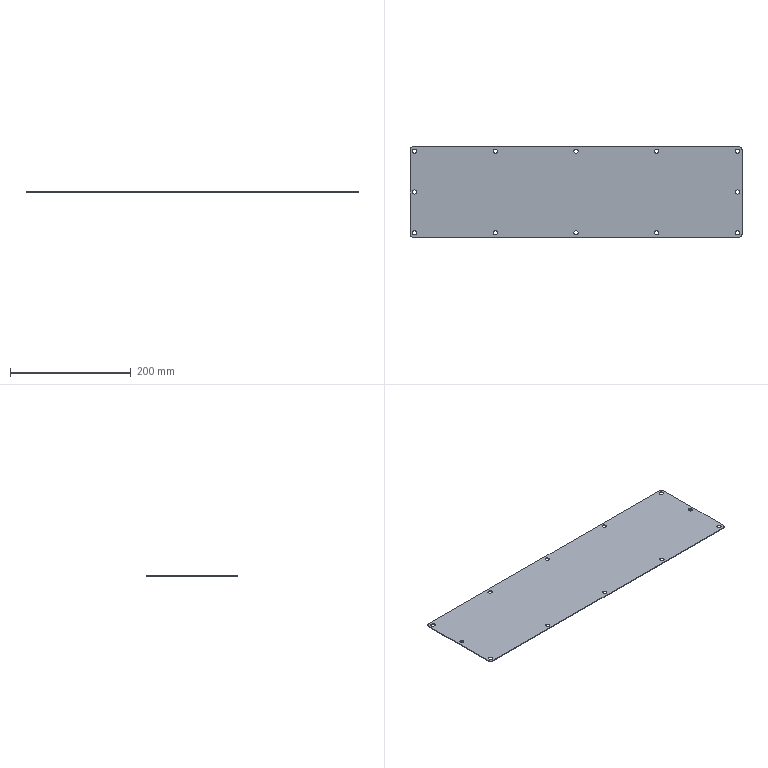Part | SolidWorks | features FlatPattern 1, SMBaseFlange 1, SheetMetal 1 | 1 solid | 34 faces | box 550 x 150 x 1.2 mm | volume 98420 mm3 | cylinder 28 | plane 6 | commonest cylinder face diameters 7 x24 10 x4
STEP:
#1=CARTESIAN_POINT('',(264.,7.5,1.2));
#2=VERTEX_POINT('',#1);
#3=CARTESIAN_POINT('',(271.,7.5,1.2));
#4=VERTEX_POINT('',#3);
#5=CARTESIAN_POINT('',(267.5,7.5,1.2));
#6=DIRECTION('',(0.,0.,1.));
#7=DIRECTION('',(1.,0.,0.));
#8=AXIS2_PLACEMENT_3D('',#5,#6,#7);
#9=CIRCLE('',#8,3.5);
#10=EDGE_CURVE('',#2,#4,#9,.T.);
#11=ORIENTED_EDGE('',*,*,#10,.T.);
#12=CARTESIAN_POINT('',(271.,7.5,0.));
#13=VERTEX_POINT('',#12);
#14=CARTESIAN_POINT('',(271.,7.5,1.2));
#15=DIRECTION('',(0.,0.,-1.));
#16=VECTOR('',#15,1000.);
#17=LINE('',#14,#16);
#18=EDGE_CURVE('',#4,#13,#17,.T.);
#19=ORIENTED_EDGE('',*,*,#18,.T.);
#20=CARTESIAN_POINT('',(264.,7.5,0.));
#21=VERTEX_POINT('',#20);
#22=CARTESIAN_POINT('',(267.5,7.5,0.));
#23=DIRECTION('',(0.,0.,1.));
#24=DIRECTION('',(1.,0.,0.));
#25=AXIS2_PLACEMENT_3D('',#22,#23,#24);
#26=CIRCLE('',#25,3.5);
#27=EDGE_CURVE('',#21,#13,#26,.T.);
#28=ORIENTED_EDGE('',*,*,#27,.F.);
#29=CARTESIAN_POINT('',(264.,7.5,1.2));
#30=DIRECTION('',(0.,0.,-1.));
#31=VECTOR('',#30,1000.);
#32=LINE('',#29,#31);
#33=EDGE_CURVE('',#2,#21,#32,.T.);
#34=ORIENTED_EDGE('',*,*,#33,.F.);
#35=EDGE_LOOP('',(#11,#19,#28,#34));
#36=FACE_OUTER_BOUND('',#35,.T.);
#37=CARTESIAN_POINT('',(267.5,7.5,1.2));
#38=DIRECTION('',(0.,0.,-1.));
#39=DIRECTION('',(-1.,0.,0.));
#40=AXIS2_PLACEMENT_3D('',#37,#38,#39);
#41=CYLINDRICAL_SURFACE('',#40,3.5);
#42=ADVANCED_FACE('',(#36),#41,.F.);
#43=CARTESIAN_POINT('',(264.,142.5,1.2));
#44=VERTEX_POINT('',#43);
#45=CARTESIAN_POINT('',(271.,142.5,1.2));
#46=VERTEX_POINT('',#45);
#47=CARTESIAN_POINT('',(267.5,142.5,1.2));
#48=DIRECTION('',(0.,0.,1.));
#49=DIRECTION('',(1.,0.,0.));
#50=AXIS2_PLACEMENT_3D('',#47,#48,#49);
#51=CIRCLE('',#50,3.5);
#52=EDGE_CURVE('',#44,#46,#51,.T.);
#53=ORIENTED_EDGE('',*,*,#52,.T.);
#54=CARTESIAN_POINT('',(271.,142.5,0.));
#55=VERTEX_POINT('',#54);
#56=CARTESIAN_POINT('',(271.,142.5,1.2));
#57=DIRECTION('',(0.,0.,-1.));
#58=VECTOR('',#57,1000.);
#59=LINE('',#56,#58);
#60=EDGE_CURVE('',#46,#55,#59,.T.);
#61=ORIENTED_EDGE('',*,*,#60,.T.);
#62=CARTESIAN_POINT('',(264.,142.5,0.));
#63=VERTEX_POINT('',#62);
#64=CARTESIAN_POINT('',(267.5,142.5,0.));
#65=DIRECTION('',(0.,0.,1.));
#66=DIRECTION('',(1.,0.,0.));
#67=AXIS2_PLACEMENT_3D('',#64,#65,#66);
#68=CIRCLE('',#67,3.5);
#69=EDGE_CURVE('',#63,#55,#68,.T.);
#70=ORIENTED_EDGE('',*,*,#69,.F.);
#71=CARTESIAN_POINT('',(264.,142.5,1.2));
#72=DIRECTION('',(0.,0.,-1.));
#73=VECTOR('',#72,1000.);
#74=LINE('',#71,#73);
#75=EDGE_CURVE('',#44,#63,#74,.T.);
#76=ORIENTED_EDGE('',*,*,#75,.F.);
#77=EDGE_LOOP('',(#53,#61,#70,#76));
#78=FACE_OUTER_BOUND('',#77,.T.);
#79=CARTESIAN_POINT('',(267.5,142.5,1.2));
#80=DIRECTION('',(0.,0.,-1.));
#81=DIRECTION('',(-1.,0.,0.));
#82=AXIS2_PLACEMENT_3D('',#79,#80,#81);
#83=CYLINDRICAL_SURFACE('',#82,3.5);
#84=ADVANCED_FACE('',(#78),#83,.F.);
#85=CARTESIAN_POINT('',(130.25,7.5,1.2));
#86=VERTEX_POINT('',#85);
#87=CARTESIAN_POINT('',(137.25,7.5,1.2));
#88=VERTEX_POINT('',#87);
#89=CARTESIAN_POINT('',(133.75,7.5,1.2));
#90=DIRECTION('',(0.,0.,1.));
#91=DIRECTION('',(1.,0.,0.));
#92=AXIS2_PLACEMENT_3D('',#89,#90,#91);
#93=CIRCLE('',#92,3.5);
#94=EDGE_CURVE('',#86,#88,#93,.T.);
#95=ORIENTED_EDGE('',*,*,#94,.T.);
#96=CARTESIAN_POINT('',(137.25,7.5,0.));
#97=VERTEX_POINT('',#96);
#98=CARTESIAN_POINT('',(137.25,7.5,1.2));
#99=DIRECTION('',(0.,0.,-1.));
#100=VECTOR('',#99,1000.);
#101=LINE('',#98,#100);
#102=EDGE_CURVE('',#88,#97,#101,.T.);
#103=ORIENTED_EDGE('',*,*,#102,.T.);
#104=CARTESIAN_POINT('',(130.25,7.5,0.));
#105=VERTEX_POINT('',#104);
#106=CARTESIAN_POINT('',(133.75,7.5,0.));
#107=DIRECTION('',(0.,0.,1.));
#108=DIRECTION('',(1.,0.,0.));
#109=AXIS2_PLACEMENT_3D('',#106,#107,#108);
#110=CIRCLE('',#109,3.5);
#111=EDGE_CURVE('',#105,#97,#110,.T.);
#112=ORIENTED_EDGE('',*,*,#111,.F.);
#113=CARTESIAN_POINT('',(130.25,7.5,1.2));
#114=DIRECTION('',(0.,0.,-1.));
#115=VECTOR('',#114,1000.);
#116=LINE('',#113,#115);
#117=EDGE_CURVE('',#86,#105,#116,.T.);
#118=ORIENTED_EDGE('',*,*,#117,.F.);
#119=EDGE_LOOP('',(#95,#103,#112,#118));
#120=FACE_OUTER_BOUND('',#119,.T.);
#121=CARTESIAN_POINT('',(133.75,7.5,1.2));
#122=DIRECTION('',(0.,0.,-1.));
#123=DIRECTION('',(-1.,0.,0.));
#124=AXIS2_PLACEMENT_3D('',#121,#122,#123);
#125=CYLINDRICAL_SURFACE('',#124,3.5);
#126=ADVANCED_FACE('',(#120),#125,.F.);
#127=CARTESIAN_POINT('',(130.25,142.5,1.2));
#128=VERTEX_POINT('',#127);
#129=CARTESIAN_POINT('',(137.25,142.5,1.2));
#130=VERTEX_POINT('',#129);
#131=CARTESIAN_POINT('',(133.75,142.5,1.2));
#132=DIRECTION('',(0.,0.,1.));
#133=DIRECTION('',(1.,0.,0.));
#134=AXIS2_PLACEMENT_3D('',#131,#132,#133);
#135=CIRCLE('',#134,3.5);
#136=EDGE_CURVE('',#128,#130,#135,.T.);
#137=ORIENTED_EDGE('',*,*,#136,.T.);
#138=CARTESIAN_POINT('',(137.25,142.5,0.));
#139=VERTEX_POINT('',#138);
#140=CARTESIAN_POINT('',(137.25,142.5,1.2));
#141=DIRECTION('',(0.,0.,-1.));
#142=VECTOR('',#141,1000.);
#143=LINE('',#140,#142);
#144=EDGE_CURVE('',#130,#139,#143,.T.);
#145=ORIENTED_EDGE('',*,*,#144,.T.);
#146=CARTESIAN_POINT('',(130.25,142.5,0.));
#147=VERTEX_POINT('',#146);
#148=CARTESIAN_POINT('',(133.75,142.5,0.));
#149=DIRECTION('',(0.,0.,1.));
#150=DIRECTION('',(1.,0.,0.));
#151=AXIS2_PLACEMENT_3D('',#148,#149,#150);
#152=CIRCLE('',#151,3.5);
#153=EDGE_CURVE('',#147,#139,#152,.T.);
#154=ORIENTED_EDGE('',*,*,#153,.F.);
#155=CARTESIAN_POINT('',(130.25,142.5,1.2));
#156=DIRECTION('',(0.,0.,-1.));
#157=VECTOR('',#156,1000.);
#158=LINE('',#155,#157);
#159=EDGE_CURVE('',#128,#147,#158,.T.);
#160=ORIENTED_EDGE('',*,*,#159,.F.);
#161=EDGE_LOOP('',(#137,#145,#154,#160));
#162=FACE_OUTER_BOUND('',#161,.T.);
#163=CARTESIAN_POINT('',(133.75,142.5,1.2));
#164=DIRECTION('',(0.,0.,-1.));
#165=DIRECTION('',(-1.,0.,0.));
#166=AXIS2_PLACEMENT_3D('',#163,#164,#165);
#167=CYLINDRICAL_SURFACE('',#166,3.5);
#168=ADVANCED_FACE('',(#162),#167,.F.);
#169=CARTESIAN_POINT('',(-3.5,7.5,1.2));
#170=VERTEX_POINT('',#169);
#171=CARTESIAN_POINT('',(3.5,7.5,1.2));
#172=VERTEX_POINT('',#171);
#173=CARTESIAN_POINT('',(0.,7.5,1.2));
#174=DIRECTION('',(0.,0.,1.));
#175=DIRECTION('',(1.,0.,0.));
#176=AXIS2_PLACEMENT_3D('',#173,#174,#175);
#177=CIRCLE('',#176,3.5);
#178=EDGE_CURVE('',#170,#172,#177,.T.);
#179=ORIENTED_EDGE('',*,*,#178,.T.);
#180=CARTESIAN_POINT('',(3.5,7.5,0.));
#181=VERTEX_POINT('',#180);
#182=CARTESIAN_POINT('',(3.5,7.5,1.2));
#183=DIRECTION('',(0.,0.,-1.));
#184=VECTOR('',#183,1000.);
#185=LINE('',#182,#184);
#186=EDGE_CURVE('',#172,#181,#185,.T.);
#187=ORIENTED_EDGE('',*,*,#186,.T.);
#188=CARTESIAN_POINT('',(-3.5,7.5,0.));
#189=VERTEX_POINT('',#188);
#190=CARTESIAN_POINT('',(0.,7.5,0.));
#191=DIRECTION('',(0.,0.,1.));
#192=DIRECTION('',(1.,0.,0.));
#193=AXIS2_PLACEMENT_3D('',#190,#191,#192);
#194=CIRCLE('',#193,3.5);
#195=EDGE_CURVE('',#189,#181,#194,.T.);
#196=ORIENTED_EDGE('',*,*,#195,.F.);
#197=CARTESIAN_POINT('',(-3.5,7.5,1.2));
#198=DIRECTION('',(0.,0.,-1.));
#199=VECTOR('',#198,1000.);
#200=LINE('',#197,#199);
#201=EDGE_CURVE('',#170,#189,#200,.T.);
#202=ORIENTED_EDGE('',*,*,#201,.F.);
#203=EDGE_LOOP('',(#179,#187,#196,#202));
#204=FACE_OUTER_BOUND('',#203,.T.);
#205=CARTESIAN_POINT('',(0.,7.5,1.2));
#206=DIRECTION('',(0.,0.,-1.));
#207=DIRECTION('',(-1.,0.,0.));
#208=AXIS2_PLACEMENT_3D('',#205,#206,#207);
#209=CYLINDRICAL_SURFACE('',#208,3.5);
#210=ADVANCED_FACE('',(#204),#209,.F.);
#211=CARTESIAN_POINT('',(-3.5,142.5,1.2));
#212=VERTEX_POINT('',#211);
#213=CARTESIAN_POINT('',(3.5,142.5,1.2));
#214=VERTEX_POINT('',#213);
#215=CARTESIAN_POINT('',(0.,142.5,1.2));
#216=DIRECTION('',(0.,0.,1.));
#217=DIRECTION('',(1.,0.,0.));
#218=AXIS2_PLACEMENT_3D('',#215,#216,#217);
#219=CIRCLE('',#218,3.5);
#220=EDGE_CURVE('',#212,#214,#219,.T.);
#221=ORIENTED_EDGE('',*,*,#220,.T.);
#222=CARTESIAN_POINT('',(3.5,142.5,0.));
#223=VERTEX_POINT('',#222);
#224=CARTESIAN_POINT('',(3.5,142.5,1.2));
#225=DIRECTION('',(0.,0.,-1.));
#226=VECTOR('',#225,1000.);
#227=LINE('',#224,#226);
#228=EDGE_CURVE('',#214,#223,#227,.T.);
#229=ORIENTED_EDGE('',*,*,#228,.T.);
#230=CARTESIAN_POINT('',(-3.5,142.5,0.));
#231=VERTEX_POINT('',#230);
#232=CARTESIAN_POINT('',(0.,142.5,0.));
#233=DIRECTION('',(0.,0.,1.));
#234=DIRECTION('',(1.,0.,0.));
#235=AXIS2_PLACEMENT_3D('',#232,#233,#234);
#236=CIRCLE('',#235,3.5);
#237=EDGE_CURVE('',#231,#223,#236,.T.);
#238=ORIENTED_EDGE('',*,*,#237,.F.);
#239=CARTESIAN_POINT('',(-3.5,142.5,1.2));
#240=DIRECTION('',(0.,0.,-1.));
#241=VECTOR('',#240,1000.);
#242=LINE('',#239,#241);
#243=EDGE_CURVE('',#212,#231,#242,.T.);
#244=ORIENTED_EDGE('',*,*,#243,.F.);
#245=EDGE_LOOP('',(#221,#229,#238,#244));
#246=FACE_OUTER_BOUND('',#245,.T.);
#247=CARTESIAN_POINT('',(0.,142.5,1.2));
#248=DIRECTION('',(0.,0.,-1.));
#249=DIRECTION('',(-1.,0.,0.));
#250=AXIS2_PLACEMENT_3D('',#247,#248,#249);
#251=CYLINDRICAL_SURFACE('',#250,3.5);
#252=ADVANCED_FACE('',(#246),#251,.F.);
#253=CARTESIAN_POINT('',(-137.25,7.5,1.2));
#254=VERTEX_POINT('',#253);
#255=CARTESIAN_POINT('',(-130.25,7.5,1.2));
#256=VERTEX_POINT('',#255);
#257=CARTESIAN_POINT('',(-133.75,7.5,1.2));
#258=DIRECTION('',(0.,0.,1.));
#259=DIRECTION('',(1.,0.,0.));
#260=AXIS2_PLACEMENT_3D('',#257,#258,#259);
#261=CIRCLE('',#260,3.5);
#262=EDGE_CURVE('',#254,#256,#261,.T.);
#263=ORIENTED_EDGE('',*,*,#262,.T.);
#264=CARTESIAN_POINT('',(-130.25,7.5,0.));
#265=VERTEX_POINT('',#264);
#266=CARTESIAN_POINT('',(-130.25,7.5,1.2));
#267=DIRECTION('',(0.,0.,-1.));
#268=VECTOR('',#267,1000.);
#269=LINE('',#266,#268);
#270=EDGE_CURVE('',#256,#265,#269,.T.);
#271=ORIENTED_EDGE('',*,*,#270,.T.);
#272=CARTESIAN_POINT('',(-137.25,7.5,0.));
#273=VERTEX_POINT('',#272);
#274=CARTESIAN_POINT('',(-133.75,7.5,0.));
#275=DIRECTION('',(0.,0.,1.));
#276=DIRECTION('',(1.,0.,0.));
#277=AXIS2_PLACEMENT_3D('',#274,#275,#276);
#278=CIRCLE('',#277,3.5);
#279=EDGE_CURVE('',#273,#265,#278,.T.);
#280=ORIENTED_EDGE('',*,*,#279,.F.);
#281=CARTESIAN_POINT('',(-137.25,7.5,1.2));
#282=DIRECTION('',(0.,0.,-1.));
#283=VECTOR('',#282,1000.);
#284=LINE('',#281,#283);
#285=EDGE_CURVE('',#254,#273,#284,.T.);
#286=ORIENTED_EDGE('',*,*,#285,.F.);
#287=EDGE_LOOP('',(#263,#271,#280,#286));
#288=FACE_OUTER_BOUND('',#287,.T.);
#289=CARTESIAN_POINT('',(-133.75,7.5,1.2));
#290=DIRECTION('',(0.,0.,-1.));
#291=DIRECTION('',(-1.,0.,0.));
#292=AXIS2_PLACEMENT_3D('',#289,#290,#291);
#293=CYLINDRICAL_SURFACE('',#292,3.5);
#294=ADVANCED_FACE('',(#288),#293,.F.);
#295=CARTESIAN_POINT('',(-137.25,142.5,1.2));
#296=VERTEX_POINT('',#295);
#297=CARTESIAN_POINT('',(-130.25,142.5,1.2));
#298=VERTEX_POINT('',#297);
#299=CARTESIAN_POINT('',(-133.75,142.5,1.2));
#300=DIRECTION('',(0.,0.,1.));
#301=DIRECTION('',(1.,0.,0.));
#302=AXIS2_PLACEMENT_3D('',#299,#300,#301);
#303=CIRCLE('',#302,3.5);
#304=EDGE_CURVE('',#296,#298,#303,.T.);
#305=ORIENTED_EDGE('',*,*,#304,.T.);
#306=CARTESIAN_POINT('',(-130.25,142.5,0.));
#307=VERTEX_POINT('',#306);
#308=CARTESIAN_POINT('',(-130.25,142.5,1.2));
#309=DIRECTION('',(0.,0.,-1.));
#310=VECTOR('',#309,1000.);
#311=LINE('',#308,#310);
#312=EDGE_CURVE('',#298,#307,#311,.T.);
#313=ORIENTED_EDGE('',*,*,#312,.T.);
#314=CARTESIAN_POINT('',(-137.25,142.5,0.));
#315=VERTEX_POINT('',#314);
#316=CARTESIAN_POINT('',(-133.75,142.5,0.));
#317=DIRECTION('',(0.,0.,1.));
#318=DIRECTION('',(1.,0.,0.));
#319=AXIS2_PLACEMENT_3D('',#316,#317,#318);
#320=CIRCLE('',#319,3.5);
#321=EDGE_CURVE('',#315,#307,#320,.T.);
#322=ORIENTED_EDGE('',*,*,#321,.F.);
#323=CARTESIAN_POINT('',(-137.25,142.5,1.2));
#324=DIRECTION('',(0.,0.,-1.));
#325=VECTOR('',#324,1000.);
#326=LINE('',#323,#325);
#327=EDGE_CURVE('',#296,#315,#326,.T.);
#328=ORIENTED_EDGE('',*,*,#327,.F.);
#329=EDGE_LOOP('',(#305,#313,#322,#328));
#330=FACE_OUTER_BOUND('',#329,.T.);
#331=CARTESIAN_POINT('',(-133.75,142.5,1.2));
#332=DIRECTION('',(0.,0.,-1.));
#333=DIRECTION('',(-1.,0.,0.));
#334=AXIS2_PLACEMENT_3D('',#331,#332,#333);
#335=CYLINDRICAL_SURFACE('',#334,3.5);
#336=ADVANCED_FACE('',(#330),#335,.F.);
#337=CARTESIAN_POINT('',(264.,75.,1.2));
#338=VERTEX_POINT('',#337);
#339=CARTESIAN_POINT('',(271.,75.,1.2));
#340=VERTEX_POINT('',#339);
#341=CARTESIAN_POINT('',(267.5,75.,1.2));
#342=DIRECTION('',(0.,0.,1.));
#343=DIRECTION('',(1.,0.,0.));
#344=AXIS2_PLACEMENT_3D('',#341,#342,#343);
#345=CIRCLE('',#344,3.5);
#346=EDGE_CURVE('',#338,#340,#345,.T.);
#347=ORIENTED_EDGE('',*,*,#346,.T.);
#348=CARTESIAN_POINT('',(271.,75.,0.));
#349=VERTEX_POINT('',#348);
#350=CARTESIAN_POINT('',(271.,75.,1.2));
#351=DIRECTION('',(0.,0.,-1.));
#352=VECTOR('',#351,1000.);
#353=LINE('',#350,#352);
#354=EDGE_CURVE('',#340,#349,#353,.T.);
#355=ORIENTED_EDGE('',*,*,#354,.T.);
#356=CARTESIAN_POINT('',(264.,75.,0.));
#357=VERTEX_POINT('',#356);
#358=CARTESIAN_POINT('',(267.5,75.,0.));
#359=DIRECTION('',(0.,0.,1.));
#360=DIRECTION('',(1.,0.,0.));
#361=AXIS2_PLACEMENT_3D('',#358,#359,#360);
#362=CIRCLE('',#361,3.5);
#363=EDGE_CURVE('',#357,#349,#362,.T.);
#364=ORIENTED_EDGE('',*,*,#363,.F.);
#365=CARTESIAN_POINT('',(264.,75.,1.2));
#366=DIRECTION('',(0.,0.,-1.));
#367=VECTOR('',#366,1000.);
#368=LINE('',#365,#367);
#369=EDGE_CURVE('',#338,#357,#368,.T.);
#370=ORIENTED_EDGE('',*,*,#369,.F.);
#371=EDGE_LOOP('',(#347,#355,#364,#370));
#372=FACE_OUTER_BOUND('',#371,.T.);
#373=CARTESIAN_POINT('',(267.5,75.,1.2));
#374=DIRECTION('',(0.,0.,-1.));
#375=DIRECTION('',(-1.,0.,0.));
#376=AXIS2_PLACEMENT_3D('',#373,#374,#375);
#377=CYLINDRICAL_SURFACE('',#376,3.5);
#378=ADVANCED_FACE('',(#372),#377,.F.);
#379=CARTESIAN_POINT('',(-271.,7.5,1.2));
#380=VERTEX_POINT('',#379);
#381=CARTESIAN_POINT('',(-264.,7.5,1.2));
#382=VERTEX_POINT('',#381);
#383=CARTESIAN_POINT('',(-267.5,7.5,1.2));
#384=DIRECTION('',(0.,0.,1.));
#385=DIRECTION('',(1.,0.,0.));
#386=AXIS2_PLACEMENT_3D('',#383,#384,#385);
#387=CIRCLE('',#386,3.5);
#388=EDGE_CURVE('',#380,#382,#387,.T.);
#389=ORIENTED_EDGE('',*,*,#388,.T.);
#390=CARTESIAN_POINT('',(-264.,7.5,0.));
#391=VERTEX_POINT('',#390);
#392=CARTESIAN_POINT('',(-264.,7.5,1.2));
#393=DIRECTION('',(0.,0.,-1.));
#394=VECTOR('',#393,1000.);
#395=LINE('',#392,#394);
#396=EDGE_CURVE('',#382,#391,#395,.T.);
#397=ORIENTED_EDGE('',*,*,#396,.T.);
#398=CARTESIAN_POINT('',(-271.,7.5,0.));
#399=VERTEX_POINT('',#398);
#400=CARTESIAN_POINT('',(-267.5,7.5,0.));
#401=DIRECTION('',(0.,0.,1.));
#402=DIRECTION('',(1.,0.,0.));
#403=AXIS2_PLACEMENT_3D('',#400,#401,#402);
#404=CIRCLE('',#403,3.5);
#405=EDGE_CURVE('',#399,#391,#404,.T.);
#406=ORIENTED_EDGE('',*,*,#405,.F.);
#407=CARTESIAN_POINT('',(-271.,7.5,1.2));
#408=DIRECTION('',(0.,0.,-1.));
#409=VECTOR('',#408,1000.);
#410=LINE('',#407,#409);
#411=EDGE_CURVE('',#380,#399,#410,.T.);
#412=ORIENTED_EDGE('',*,*,#411,.F.);
#413=EDGE_LOOP('',(#389,#397,#406,#412));
#414=FACE_OUTER_BOUND('',#413,.T.);
#415=CARTESIAN_POINT('',(-267.5,7.5,1.2));
#416=DIRECTION('',(0.,0.,-1.));
#417=DIRECTION('',(-1.,0.,0.));
#418=AXIS2_PLACEMENT_3D('',#415,#416,#417);
#419=CYLINDRICAL_SURFACE('',#418,3.5);
#420=ADVANCED_FACE('',(#414),#419,.F.);
#421=CARTESIAN_POINT('',(-271.,142.5,1.2));
#422=VERTEX_POINT('',#421);
#423=CARTESIAN_POINT('',(-264.,142.5,1.2));
#424=VERTEX_POINT('',#423);
#425=CARTESIAN_POINT('',(-267.5,142.5,1.2));
#426=DIRECTION('',(0.,0.,1.));
#427=DIRECTION('',(1.,0.,0.));
#428=AXIS2_PLACEMENT_3D('',#425,#426,#427);
#429=CIRCLE('',#428,3.5);
#430=EDGE_CURVE('',#422,#424,#429,.T.);
#431=ORIENTED_EDGE('',*,*,#430,.T.);
#432=CARTESIAN_POINT('',(-264.,142.5,0.));
#433=VERTEX_POINT('',#432);
#434=CARTESIAN_POINT('',(-264.,142.5,1.2));
#435=DIRECTION('',(0.,0.,-1.));
#436=VECTOR('',#435,1000.);
#437=LINE('',#434,#436);
#438=EDGE_CURVE('',#424,#433,#437,.T.);
#439=ORIENTED_EDGE('',*,*,#438,.T.);
#440=CARTESIAN_POINT('',(-271.,142.5,0.));
#441=VERTEX_POINT('',#440);
#442=CARTESIAN_POINT('',(-267.5,142.5,0.));
#443=DIRECTION('',(0.,0.,1.));
#444=DIRECTION('',(1.,0.,0.));
#445=AXIS2_PLACEMENT_3D('',#442,#443,#444);
#446=CIRCLE('',#445,3.5);
#447=EDGE_CURVE('',#441,#433,#446,.T.);
#448=ORIENTED_EDGE('',*,*,#447,.F.);
#449=CARTESIAN_POINT('',(-271.,142.5,1.2));
#450=DIRECTION('',(0.,0.,-1.));
#451=VECTOR('',#450,1000.);
#452=LINE('',#449,#451);
#453=EDGE_CURVE('',#422,#441,#452,.T.);
#454=ORIENTED_EDGE('',*,*,#453,.F.);
#455=EDGE_LOOP('',(#431,#439,#448,#454));
#456=FACE_OUTER_BOUND('',#455,.T.);
#457=CARTESIAN_POINT('',(-267.5,142.5,1.2));
#458=DIRECTION('',(0.,0.,-1.));
#459=DIRECTION('',(-1.,0.,0.));
#460=AXIS2_PLACEMENT_3D('',#457,#458,#459);
#461=CYLINDRICAL_SURFACE('',#460,3.5);
#462=ADVANCED_FACE('',(#456),#461,.F.);
#463=CARTESIAN_POINT('',(-271.,75.,1.2));
#464=VERTEX_POINT('',#463);
#465=CARTESIAN_POINT('',(-264.,75.,1.2));
#466=VERTEX_POINT('',#465);
#467=CARTESIAN_POINT('',(-267.5,75.,1.2));
#468=DIRECTION('',(0.,0.,1.));
#469=DIRECTION('',(1.,0.,0.));
#470=AXIS2_PLACEMENT_3D('',#467,#468,#469);
#471=CIRCLE('',#470,3.5);
#472=EDGE_CURVE('',#464,#466,#471,.T.);
#473=ORIENTED_EDGE('',*,*,#472,.T.);
#474=CARTESIAN_POINT('',(-264.,75.,0.));
#475=VERTEX_POINT('',#474);
#476=CARTESIAN_POINT('',(-264.,75.,1.2));
#477=DIRECTION('',(0.,0.,-1.));
#478=VECTOR('',#477,1000.);
#479=LINE('',#476,#478);
#480=EDGE_CURVE('',#466,#475,#479,.T.);
#481=ORIENTED_EDGE('',*,*,#480,.T.);
#482=CARTESIAN_POINT('',(-271.,75.,0.));
#483=VERTEX_POINT('',#482);
#484=CARTESIAN_POINT('',(-267.5,75.,0.));
#485=DIRECTION('',(0.,0.,1.));
#486=DIRECTION('',(1.,0.,0.));
#487=AXIS2_PLACEMENT_3D('',#484,#485,#486);
#488=CIRCLE('',#487,3.5);
#489=EDGE_CURVE('',#483,#475,#488,.T.);
#490=ORIENTED_EDGE('',*,*,#489,.F.);
#491=CARTESIAN_POINT('',(-271.,75.,1.2));
#492=DIRECTION('',(0.,0.,-1.));
#493=VECTOR('',#492,1000.);
#494=LINE('',#491,#493);
#495=EDGE_CURVE('',#464,#483,#494,.T.);
#496=ORIENTED_EDGE('',*,*,#495,.F.);
#497=EDGE_LOOP('',(#473,#481,#490,#496));
#498=FACE_OUTER_BOUND('',#497,.T.);
#499=CARTESIAN_POINT('',(-267.5,75.,1.2));
#500=DIRECTION('',(0.,0.,-1.));
#501=DIRECTION('',(-1.,0.,0.));
#502=AXIS2_PLACEMENT_3D('',#499,#500,#501);
#503=CYLINDRICAL_SURFACE('',#502,3.5);
#504=ADVANCED_FACE('',(#498),#503,.F.);
#505=ORIENTED_EDGE('',*,*,#52,.F.);
#506=CARTESIAN_POINT('',(267.5,142.5,1.2));
#507=DIRECTION('',(0.,0.,1.));
#508=DIRECTION('',(1.,0.,0.));
#509=AXIS2_PLACEMENT_3D('',#506,#507,#508);
#510=CIRCLE('',#509,3.5);
#511=EDGE_CURVE('',#46,#44,#510,.T.);
#512=ORIENTED_EDGE('',*,*,#511,.F.);
#513=EDGE_LOOP('',(#505,#512));
#514=FACE_BOUND('',#513,.T.);
#515=ORIENTED_EDGE('',*,*,#136,.F.);
#516=CARTESIAN_POINT('',(133.75,142.5,1.2));
#517=DIRECTION('',(0.,0.,1.));
#518=DIRECTION('',(1.,0.,0.));
#519=AXIS2_PLACEMENT_3D('',#516,#517,#518);
#520=CIRCLE('',#519,3.5);
#521=EDGE_CURVE('',#130,#128,#520,.T.);
#522=ORIENTED_EDGE('',*,*,#521,.F.);
#523=EDGE_LOOP('',(#515,#522));
#524=FACE_BOUND('',#523,.T.);
#525=ORIENTED_EDGE('',*,*,#220,.F.);
#526=CARTESIAN_POINT('',(0.,142.5,1.2));
#527=DIRECTION('',(0.,0.,1.));
#528=DIRECTION('',(1.,0.,0.));
#529=AXIS2_PLACEMENT_3D('',#526,#527,#528);
#530=CIRCLE('',#529,3.5);
#531=EDGE_CURVE('',#214,#212,#530,.T.);
#532=ORIENTED_EDGE('',*,*,#531,.F.);
#533=EDGE_LOOP('',(#525,#532));
#534=FACE_BOUND('',#533,.T.);
#535=ORIENTED_EDGE('',*,*,#304,.F.);
#536=CARTESIAN_POINT('',(-133.75,142.5,1.2));
#537=DIRECTION('',(0.,0.,1.));
#538=DIRECTION('',(1.,0.,0.));
#539=AXIS2_PLACEMENT_3D('',#536,#537,#538);
#540=CIRCLE('',#539,3.5);
#541=EDGE_CURVE('',#298,#296,#540,.T.);
#542=ORIENTED_EDGE('',*,*,#541,.F.);
#543=EDGE_LOOP('',(#535,#542));
#544=FACE_BOUND('',#543,.T.);
#545=ORIENTED_EDGE('',*,*,#388,.F.);
#546=CARTESIAN_POINT('',(-267.5,7.5,1.2));
#547=DIRECTION('',(0.,0.,1.));
#548=DIRECTION('',(1.,0.,0.));
#549=AXIS2_PLACEMENT_3D('',#546,#547,#548);
#550=CIRCLE('',#549,3.5);
#551=EDGE_CURVE('',#382,#380,#550,.T.);
#552=ORIENTED_EDGE('',*,*,#551,.F.);
#553=EDGE_LOOP('',(#545,#552));
#554=FACE_BOUND('',#553,.T.);
#555=ORIENTED_EDGE('',*,*,#472,.F.);
#556=CARTESIAN_POINT('',(-267.5,75.,1.2));
#557=DIRECTION('',(0.,0.,1.));
#558=DIRECTION('',(1.,0.,0.));
#559=AXIS2_PLACEMENT_3D('',#556,#557,#558);
#560=CIRCLE('',#559,3.5);
#561=EDGE_CURVE('',#466,#464,#560,.T.);
#562=ORIENTED_EDGE('',*,*,#561,.F.);
#563=EDGE_LOOP('',(#555,#562));
#564=FACE_BOUND('',#563,.T.);
#565=CARTESIAN_POINT('',(270.,0.,1.2));
#566=VERTEX_POINT('',#565);
#567=CARTESIAN_POINT('',(275.,5.,1.2));
#568=VERTEX_POINT('',#567);
#569=CARTESIAN_POINT('',(270.,5.,1.2));
#570=DIRECTION('',(0.,0.,1.));
#571=DIRECTION('',(1.,0.,0.));
#572=AXIS2_PLACEMENT_3D('',#569,#570,#571);
#573=CIRCLE('',#572,5.);
#574=EDGE_CURVE('',#566,#568,#573,.T.);
#575=ORIENTED_EDGE('',*,*,#574,.T.);
#576=CARTESIAN_POINT('',(275.,145.,1.2));
#577=VERTEX_POINT('',#576);
#578=CARTESIAN_POINT('',(275.,145.,1.2));
#579=DIRECTION('',(0.,1.,0.));
#580=VECTOR('',#579,1000.);
#581=LINE('',#578,#580);
#582=EDGE_CURVE('',#568,#577,#581,.T.);
#583=ORIENTED_EDGE('',*,*,#582,.T.);
#584=CARTESIAN_POINT('',(270.,150.,1.2));
#585=VERTEX_POINT('',#584);
#586=CARTESIAN_POINT('',(270.,145.,1.2));
#587=DIRECTION('',(0.,0.,1.));
#588=DIRECTION('',(-1.,0.,0.));
#589=AXIS2_PLACEMENT_3D('',#586,#587,#588);
#590=CIRCLE('',#589,5.);
#591=EDGE_CURVE('',#577,#585,#590,.T.);
#592=ORIENTED_EDGE('',*,*,#591,.T.);
#593=CARTESIAN_POINT('',(-270.,150.,1.2));
#594=VERTEX_POINT('',#593);
#595=CARTESIAN_POINT('',(-270.,150.,1.2));
#596=DIRECTION('',(-1.,0.,0.));
#597=VECTOR('',#596,1000.);
#598=LINE('',#595,#597);
#599=EDGE_CURVE('',#585,#594,#598,.T.);
#600=ORIENTED_EDGE('',*,*,#599,.T.);
#601=CARTESIAN_POINT('',(-275.,145.,1.2));
#602=VERTEX_POINT('',#601);
#603=CARTESIAN_POINT('',(-270.,145.,1.2));
#604=DIRECTION('',(0.,0.,1.));
#605=DIRECTION('',(-1.,0.,0.));
#606=AXIS2_PLACEMENT_3D('',#603,#604,#605);
#607=CIRCLE('',#606,5.);
#608=EDGE_CURVE('',#594,#602,#607,.T.);
#609=ORIENTED_EDGE('',*,*,#608,.T.);
#610=CARTESIAN_POINT('',(-275.,5.,1.2));
#611=VERTEX_POINT('',#610);
#612=CARTESIAN_POINT('',(-275.,5.,1.2));
#613=DIRECTION('',(0.,-1.,0.));
#614=VECTOR('',#613,1000.);
#615=LINE('',#612,#614);
#616=EDGE_CURVE('',#602,#611,#615,.T.);
#617=ORIENTED_EDGE('',*,*,#616,.T.);
#618=CARTESIAN_POINT('',(-270.,0.,1.2));
#619=VERTEX_POINT('',#618);
#620=CARTESIAN_POINT('',(-270.,5.,1.2));
#621=DIRECTION('',(0.,0.,1.));
#622=DIRECTION('',(-1.,0.,0.));
#623=AXIS2_PLACEMENT_3D('',#620,#621,#622);
#624=CIRCLE('',#623,5.);
#625=EDGE_CURVE('',#611,#619,#624,.T.);
#626=ORIENTED_EDGE('',*,*,#625,.T.);
#627=CARTESIAN_POINT('',(-270.,0.,1.2));
#628=DIRECTION('',(1.,0.,0.));
#629=VECTOR('',#628,1000.);
#630=LINE('',#627,#629);
#631=EDGE_CURVE('',#619,#566,#630,.T.);
#632=ORIENTED_EDGE('',*,*,#631,.T.);
#633=EDGE_LOOP('',(#575,#583,#592,#600,#609,#617,#626,#632));
#634=FACE_OUTER_BOUND('',#633,.T.);
#635=ORIENTED_EDGE('',*,*,#430,.F.);
#636=CARTESIAN_POINT('',(-267.5,142.5,1.2));
#637=DIRECTION('',(0.,0.,1.));
#638=DIRECTION('',(1.,0.,0.));
#639=AXIS2_PLACEMENT_3D('',#636,#637,#638);
#640=CIRCLE('',#639,3.5);
#641=EDGE_CURVE('',#424,#422,#640,.T.);
#642=ORIENTED_EDGE('',*,*,#641,.F.);
#643=EDGE_LOOP('',(#635,#642));
#644=FACE_BOUND('',#643,.T.);
#645=ORIENTED_EDGE('',*,*,#346,.F.);
#646=CARTESIAN_POINT('',(267.5,75.,1.2));
#647=DIRECTION('',(0.,0.,1.));
#648=DIRECTION('',(1.,0.,0.));
#649=AXIS2_PLACEMENT_3D('',#646,#647,#648);
#650=CIRCLE('',#649,3.5);
#651=EDGE_CURVE('',#340,#338,#650,.T.);
#652=ORIENTED_EDGE('',*,*,#651,.F.);
#653=EDGE_LOOP('',(#645,#652));
#654=FACE_BOUND('',#653,.T.);
#655=ORIENTED_EDGE('',*,*,#262,.F.);
#656=CARTESIAN_POINT('',(-133.75,7.5,1.2));
#657=DIRECTION('',(0.,0.,1.));
#658=DIRECTION('',(1.,0.,0.));
#659=AXIS2_PLACEMENT_3D('',#656,#657,#658);
#660=CIRCLE('',#659,3.5);
#661=EDGE_CURVE('',#256,#254,#660,.T.);
#662=ORIENTED_EDGE('',*,*,#661,.F.);
#663=EDGE_LOOP('',(#655,#662));
#664=FACE_BOUND('',#663,.T.);
#665=ORIENTED_EDGE('',*,*,#178,.F.);
#666=CARTESIAN_POINT('',(0.,7.5,1.2));
#667=DIRECTION('',(0.,0.,1.));
#668=DIRECTION('',(1.,0.,0.));
#669=AXIS2_PLACEMENT_3D('',#666,#667,#668);
#670=CIRCLE('',#669,3.5);
#671=EDGE_CURVE('',#172,#170,#670,.T.);
#672=ORIENTED_EDGE('',*,*,#671,.F.);
#673=EDGE_LOOP('',(#665,#672));
#674=FACE_BOUND('',#673,.T.);
#675=ORIENTED_EDGE('',*,*,#94,.F.);
#676=CARTESIAN_POINT('',(133.75,7.5,1.2));
#677=DIRECTION('',(0.,0.,1.));
#678=DIRECTION('',(1.,0.,0.));
#679=AXIS2_PLACEMENT_3D('',#676,#677,#678);
#680=CIRCLE('',#679,3.5);
#681=EDGE_CURVE('',#88,#86,#680,.T.);
#682=ORIENTED_EDGE('',*,*,#681,.F.);
#683=EDGE_LOOP('',(#675,#682));
#684=FACE_BOUND('',#683,.T.);
#685=ORIENTED_EDGE('',*,*,#10,.F.);
#686=CARTESIAN_POINT('',(267.5,7.5,1.2));
#687=DIRECTION('',(0.,0.,1.));
#688=DIRECTION('',(1.,0.,0.));
#689=AXIS2_PLACEMENT_3D('',#686,#687,#688);
#690=CIRCLE('',#689,3.5);
#691=EDGE_CURVE('',#4,#2,#690,.T.);
#692=ORIENTED_EDGE('',*,*,#691,.F.);
#693=EDGE_LOOP('',(#685,#692));
#694=FACE_BOUND('',#693,.T.);
#695=CARTESIAN_POINT('',(270.,5.,1.2));
#696=DIRECTION('',(0.,0.,1.));
#697=DIRECTION('',(1.,0.,0.));
#698=AXIS2_PLACEMENT_3D('',#695,#696,#697);
#699=PLANE('',#698);
#700=ADVANCED_FACE('',(#514,#524,#534,#544,#554,#564,#634,#644,#654,#664,#674,#684,#694),#699,.T.);
#701=CARTESIAN_POINT('',(270.,0.,0.));
#702=VERTEX_POINT('',#701);
#703=CARTESIAN_POINT('',(275.,5.,0.));
#704=VERTEX_POINT('',#703);
#705=CARTESIAN_POINT('',(270.,5.,0.));
#706=DIRECTION('',(0.,0.,1.));
#707=DIRECTION('',(1.,0.,0.));
#708=AXIS2_PLACEMENT_3D('',#705,#706,#707);
#709=CIRCLE('',#708,5.);
#710=EDGE_CURVE('',#702,#704,#709,.T.);
#711=ORIENTED_EDGE('',*,*,#710,.F.);
#712=CARTESIAN_POINT('',(-270.,0.,0.));
#713=VERTEX_POINT('',#712);
#714=CARTESIAN_POINT('',(-270.,0.,0.));
#715=DIRECTION('',(1.,0.,0.));
#716=VECTOR('',#715,1000.);
#717=LINE('',#714,#716);
#718=EDGE_CURVE('',#713,#702,#717,.T.);
#719=ORIENTED_EDGE('',*,*,#718,.F.);
#720=CARTESIAN_POINT('',(-275.,5.,0.));
#721=VERTEX_POINT('',#720);
#722=CARTESIAN_POINT('',(-270.,5.,0.));
#723=DIRECTION('',(0.,0.,1.));
#724=DIRECTION('',(-1.,0.,0.));
#725=AXIS2_PLACEMENT_3D('',#722,#723,#724);
#726=CIRCLE('',#725,5.);
#727=EDGE_CURVE('',#721,#713,#726,.T.);
#728=ORIENTED_EDGE('',*,*,#727,.F.);
#729=CARTESIAN_POINT('',(-275.,145.,0.));
#730=VERTEX_POINT('',#729);
#731=CARTESIAN_POINT('',(-275.,5.,0.));
#732=DIRECTION('',(0.,-1.,0.));
#733=VECTOR('',#732,1000.);
#734=LINE('',#731,#733);
#735=EDGE_CURVE('',#730,#721,#734,.T.);
#736=ORIENTED_EDGE('',*,*,#735,.F.);
#737=CARTESIAN_POINT('',(-270.,150.,0.));
#738=VERTEX_POINT('',#737);
#739=CARTESIAN_POINT('',(-270.,145.,0.));
#740=DIRECTION('',(0.,0.,1.));
#741=DIRECTION('',(-1.,0.,0.));
#742=AXIS2_PLACEMENT_3D('',#739,#740,#741);
#743=CIRCLE('',#742,5.);
#744=EDGE_CURVE('',#738,#730,#743,.T.);
#745=ORIENTED_EDGE('',*,*,#744,.F.);
#746=CARTESIAN_POINT('',(270.,150.,0.));
#747=VERTEX_POINT('',#746);
#748=CARTESIAN_POINT('',(-270.,150.,0.));
#749=DIRECTION('',(-1.,0.,0.));
#750=VECTOR('',#749,1000.);
#751=LINE('',#748,#750);
#752=EDGE_CURVE('',#747,#738,#751,.T.);
#753=ORIENTED_EDGE('',*,*,#752,.F.);
#754=CARTESIAN_POINT('',(275.,145.,0.));
#755=VERTEX_POINT('',#754);
#756=CARTESIAN_POINT('',(270.,145.,0.));
#757=DIRECTION('',(0.,0.,1.));
#758=DIRECTION('',(-1.,0.,0.));
#759=AXIS2_PLACEMENT_3D('',#756,#757,#758);
#760=CIRCLE('',#759,5.);
#761=EDGE_CURVE('',#755,#747,#760,.T.);
#762=ORIENTED_EDGE('',*,*,#761,.F.);
#763=CARTESIAN_POINT('',(275.,145.,0.));
#764=DIRECTION('',(0.,1.,0.));
#765=VECTOR('',#764,1000.);
#766=LINE('',#763,#765);
#767=EDGE_CURVE('',#704,#755,#766,.T.);
#768=ORIENTED_EDGE('',*,*,#767,.F.);
#769=EDGE_LOOP('',(#711,#719,#728,#736,#745,#753,#762,#768));
#770=FACE_OUTER_BOUND('',#769,.T.);
#771=ORIENTED_EDGE('',*,*,#489,.T.);
#772=CARTESIAN_POINT('',(-267.5,75.,0.));
#773=DIRECTION('',(0.,0.,1.));
#774=DIRECTION('',(1.,0.,0.));
#775=AXIS2_PLACEMENT_3D('',#772,#773,#774);
#776=CIRCLE('',#775,3.5);
#777=EDGE_CURVE('',#475,#483,#776,.T.);
#778=ORIENTED_EDGE('',*,*,#777,.T.);
#779=EDGE_LOOP('',(#771,#778));
#780=FACE_BOUND('',#779,.T.);
#781=ORIENTED_EDGE('',*,*,#447,.T.);
#782=CARTESIAN_POINT('',(-267.5,142.5,0.));
#783=DIRECTION('',(0.,0.,1.));
#784=DIRECTION('',(1.,0.,0.));
#785=AXIS2_PLACEMENT_3D('',#782,#783,#784);
#786=CIRCLE('',#785,3.5);
#787=EDGE_CURVE('',#433,#441,#786,.T.);
#788=ORIENTED_EDGE('',*,*,#787,.T.);
#789=EDGE_LOOP('',(#781,#788));
#790=FACE_BOUND('',#789,.T.);
#791=ORIENTED_EDGE('',*,*,#405,.T.);
#792=CARTESIAN_POINT('',(-267.5,7.5,0.));
#793=DIRECTION('',(0.,0.,1.));
#794=DIRECTION('',(1.,0.,0.));
#795=AXIS2_PLACEMENT_3D('',#792,#793,#794);
#796=CIRCLE('',#795,3.5);
#797=EDGE_CURVE('',#391,#399,#796,.T.);
#798=ORIENTED_EDGE('',*,*,#797,.T.);
#799=EDGE_LOOP('',(#791,#798));
#800=FACE_BOUND('',#799,.T.);
#801=ORIENTED_EDGE('',*,*,#363,.T.);
#802=CARTESIAN_POINT('',(267.5,75.,0.));
#803=DIRECTION('',(0.,0.,1.));
#804=DIRECTION('',(1.,0.,0.));
#805=AXIS2_PLACEMENT_3D('',#802,#803,#804);
#806=CIRCLE('',#805,3.5);
#807=EDGE_CURVE('',#349,#357,#806,.T.);
#808=ORIENTED_EDGE('',*,*,#807,.T.);
#809=EDGE_LOOP('',(#801,#808));
#810=FACE_BOUND('',#809,.T.);
#811=ORIENTED_EDGE('',*,*,#321,.T.);
#812=CARTESIAN_POINT('',(-133.75,142.5,0.));
#813=DIRECTION('',(0.,0.,1.));
#814=DIRECTION('',(1.,0.,0.));
#815=AXIS2_PLACEMENT_3D('',#812,#813,#814);
#816=CIRCLE('',#815,3.5);
#817=EDGE_CURVE('',#307,#315,#816,.T.);
#818=ORIENTED_EDGE('',*,*,#817,.T.);
#819=EDGE_LOOP('',(#811,#818));
#820=FACE_BOUND('',#819,.T.);
#821=ORIENTED_EDGE('',*,*,#279,.T.);
#822=CARTESIAN_POINT('',(-133.75,7.5,0.));
#823=DIRECTION('',(0.,0.,1.));
#824=DIRECTION('',(1.,0.,0.));
#825=AXIS2_PLACEMENT_3D('',#822,#823,#824);
#826=CIRCLE('',#825,3.5);
#827=EDGE_CURVE('',#265,#273,#826,.T.);
#828=ORIENTED_EDGE('',*,*,#827,.T.);
#829=EDGE_LOOP('',(#821,#828));
#830=FACE_BOUND('',#829,.T.);
#831=ORIENTED_EDGE('',*,*,#237,.T.);
#832=CARTESIAN_POINT('',(0.,142.5,0.));
#833=DIRECTION('',(0.,0.,1.));
#834=DIRECTION('',(1.,0.,0.));
#835=AXIS2_PLACEMENT_3D('',#832,#833,#834);
#836=CIRCLE('',#835,3.5);
#837=EDGE_CURVE('',#223,#231,#836,.T.);
#838=ORIENTED_EDGE('',*,*,#837,.T.);
#839=EDGE_LOOP('',(#831,#838));
#840=FACE_BOUND('',#839,.T.);
#841=ORIENTED_EDGE('',*,*,#195,.T.);
#842=CARTESIAN_POINT('',(0.,7.5,0.));
#843=DIRECTION('',(0.,0.,1.));
#844=DIRECTION('',(1.,0.,0.));
#845=AXIS2_PLACEMENT_3D('',#842,#843,#844);
#846=CIRCLE('',#845,3.5);
#847=EDGE_CURVE('',#181,#189,#846,.T.);
#848=ORIENTED_EDGE('',*,*,#847,.T.);
#849=EDGE_LOOP('',(#841,#848));
#850=FACE_BOUND('',#849,.T.);
#851=ORIENTED_EDGE('',*,*,#153,.T.);
#852=CARTESIAN_POINT('',(133.75,142.5,0.));
#853=DIRECTION('',(0.,0.,1.));
#854=DIRECTION('',(1.,0.,0.));
#855=AXIS2_PLACEMENT_3D('',#852,#853,#854);
#856=CIRCLE('',#855,3.5);
#857=EDGE_CURVE('',#139,#147,#856,.T.);
#858=ORIENTED_EDGE('',*,*,#857,.T.);
#859=EDGE_LOOP('',(#851,#858));
#860=FACE_BOUND('',#859,.T.);
#861=ORIENTED_EDGE('',*,*,#111,.T.);
#862=CARTESIAN_POINT('',(133.75,7.5,0.));
#863=DIRECTION('',(0.,0.,1.));
#864=DIRECTION('',(1.,0.,0.));
#865=AXIS2_PLACEMENT_3D('',#862,#863,#864);
#866=CIRCLE('',#865,3.5);
#867=EDGE_CURVE('',#97,#105,#866,.T.);
#868=ORIENTED_EDGE('',*,*,#867,.T.);
#869=EDGE_LOOP('',(#861,#868));
#870=FACE_BOUND('',#869,.T.);
#871=ORIENTED_EDGE('',*,*,#69,.T.);
#872=CARTESIAN_POINT('',(267.5,142.5,0.));
#873=DIRECTION('',(0.,0.,1.));
#874=DIRECTION('',(1.,0.,0.));
#875=AXIS2_PLACEMENT_3D('',#872,#873,#874);
#876=CIRCLE('',#875,3.5);
#877=EDGE_CURVE('',#55,#63,#876,.T.);
#878=ORIENTED_EDGE('',*,*,#877,.T.);
#879=EDGE_LOOP('',(#871,#878));
#880=FACE_BOUND('',#879,.T.);
#881=ORIENTED_EDGE('',*,*,#27,.T.);
#882=CARTESIAN_POINT('',(267.5,7.5,0.));
#883=DIRECTION('',(0.,0.,1.));
#884=DIRECTION('',(1.,0.,0.));
#885=AXIS2_PLACEMENT_3D('',#882,#883,#884);
#886=CIRCLE('',#885,3.5);
#887=EDGE_CURVE('',#13,#21,#886,.T.);
#888=ORIENTED_EDGE('',*,*,#887,.T.);
#889=EDGE_LOOP('',(#881,#888));
#890=FACE_BOUND('',#889,.T.);
#891=CARTESIAN_POINT('',(270.,5.,0.));
#892=DIRECTION('',(0.,0.,1.));
#893=DIRECTION('',(1.,0.,0.));
#894=AXIS2_PLACEMENT_3D('',#891,#892,#893);
#895=PLANE('',#894);
#896=ADVANCED_FACE('',(#770,#780,#790,#800,#810,#820,#830,#840,#850,#860,#870,#880,#890),#895,.F.);
#897=ORIENTED_EDGE('',*,*,#710,.T.);
#898=CARTESIAN_POINT('',(275.,5.,1.2));
#899=DIRECTION('',(0.,0.,-1.));
#900=VECTOR('',#899,1000.);
#901=LINE('',#898,#900);
#902=EDGE_CURVE('',#568,#704,#901,.T.);
#903=ORIENTED_EDGE('',*,*,#902,.F.);
#904=ORIENTED_EDGE('',*,*,#574,.F.);
#905=CARTESIAN_POINT('',(270.,0.,1.2));
#906=DIRECTION('',(0.,0.,-1.));
#907=VECTOR('',#906,1000.);
#908=LINE('',#905,#907);
#909=EDGE_CURVE('',#566,#702,#908,.T.);
#910=ORIENTED_EDGE('',*,*,#909,.T.);
#911=EDGE_LOOP('',(#897,#903,#904,#910));
#912=FACE_OUTER_BOUND('',#911,.T.);
#913=CARTESIAN_POINT('',(270.,5.,1.2));
#914=DIRECTION('',(0.,0.,-1.));
#915=DIRECTION('',(-1.,0.,0.));
#916=AXIS2_PLACEMENT_3D('',#913,#914,#915);
#917=CYLINDRICAL_SURFACE('',#916,5.);
#918=ADVANCED_FACE('',(#912),#917,.T.);
#919=ORIENTED_EDGE('',*,*,#767,.T.);
#920=CARTESIAN_POINT('',(275.,145.,1.2));
#921=DIRECTION('',(0.,0.,-1.));
#922=VECTOR('',#921,1000.);
#923=LINE('',#920,#922);
#924=EDGE_CURVE('',#577,#755,#923,.T.);
#925=ORIENTED_EDGE('',*,*,#924,.F.);
#926=ORIENTED_EDGE('',*,*,#582,.F.);
#927=ORIENTED_EDGE('',*,*,#902,.T.);
#928=EDGE_LOOP('',(#919,#925,#926,#927));
#929=FACE_OUTER_BOUND('',#928,.T.);
#930=CARTESIAN_POINT('',(275.,145.,1.2));
#931=DIRECTION('',(-1.,0.,0.));
#932=DIRECTION('',(0.,0.,1.));
#933=AXIS2_PLACEMENT_3D('',#930,#931,#932);
#934=PLANE('',#933);
#935=ADVANCED_FACE('',(#929),#934,.F.);
#936=ORIENTED_EDGE('',*,*,#761,.T.);
#937=CARTESIAN_POINT('',(270.,150.,1.2));
#938=DIRECTION('',(0.,0.,-1.));
#939=VECTOR('',#938,1000.);
#940=LINE('',#937,#939);
#941=EDGE_CURVE('',#585,#747,#940,.T.);
#942=ORIENTED_EDGE('',*,*,#941,.F.);
#943=ORIENTED_EDGE('',*,*,#591,.F.);
#944=ORIENTED_EDGE('',*,*,#924,.T.);
#945=EDGE_LOOP('',(#936,#942,#943,#944));
#946=FACE_OUTER_BOUND('',#945,.T.);
#947=CARTESIAN_POINT('',(270.,145.,1.2));
#948=DIRECTION('',(0.,0.,-1.));
#949=DIRECTION('',(-1.,0.,0.));
#950=AXIS2_PLACEMENT_3D('',#947,#948,#949);
#951=CYLINDRICAL_SURFACE('',#950,5.);
#952=ADVANCED_FACE('',(#946),#951,.T.);
#953=ORIENTED_EDGE('',*,*,#752,.T.);
#954=CARTESIAN_POINT('',(-270.,150.,1.2));
#955=DIRECTION('',(0.,0.,-1.));
#956=VECTOR('',#955,1000.);
#957=LINE('',#954,#956);
#958=EDGE_CURVE('',#594,#738,#957,.T.);
#959=ORIENTED_EDGE('',*,*,#958,.F.);
#960=ORIENTED_EDGE('',*,*,#599,.F.);
#961=ORIENTED_EDGE('',*,*,#941,.T.);
#962=EDGE_LOOP('',(#953,#959,#960,#961));
#963=FACE_OUTER_BOUND('',#962,.T.);
#964=CARTESIAN_POINT('',(-270.,150.,1.2));
#965=DIRECTION('',(0.,-1.,0.));
#966=DIRECTION('',(0.,0.,-1.));
#967=AXIS2_PLACEMENT_3D('',#964,#965,#966);
#968=PLANE('',#967);
#969=ADVANCED_FACE('',(#963),#968,.F.);
#970=ORIENTED_EDGE('',*,*,#744,.T.);
#971=CARTESIAN_POINT('',(-275.,145.,1.2));
#972=DIRECTION('',(0.,0.,-1.));
#973=VECTOR('',#972,1000.);
#974=LINE('',#971,#973);
#975=EDGE_CURVE('',#602,#730,#974,.T.);
#976=ORIENTED_EDGE('',*,*,#975,.F.);
#977=ORIENTED_EDGE('',*,*,#608,.F.);
#978=ORIENTED_EDGE('',*,*,#958,.T.);
#979=EDGE_LOOP('',(#970,#976,#977,#978));
#980=FACE_OUTER_BOUND('',#979,.T.);
#981=CARTESIAN_POINT('',(-270.,145.,1.2));
#982=DIRECTION('',(0.,0.,-1.));
#983=DIRECTION('',(-1.,0.,0.));
#984=AXIS2_PLACEMENT_3D('',#981,#982,#983);
#985=CYLINDRICAL_SURFACE('',#984,5.);
#986=ADVANCED_FACE('',(#980),#985,.T.);
#987=ORIENTED_EDGE('',*,*,#735,.T.);
#988=CARTESIAN_POINT('',(-275.,5.,1.2));
#989=DIRECTION('',(0.,0.,-1.));
#990=VECTOR('',#989,1000.);
#991=LINE('',#988,#990);
#992=EDGE_CURVE('',#611,#721,#991,.T.);
#993=ORIENTED_EDGE('',*,*,#992,.F.);
#994=ORIENTED_EDGE('',*,*,#616,.F.);
#995=ORIENTED_EDGE('',*,*,#975,.T.);
#996=EDGE_LOOP('',(#987,#993,#994,#995));
#997=FACE_OUTER_BOUND('',#996,.T.);
#998=CARTESIAN_POINT('',(-275.,5.,1.2));
#999=DIRECTION('',(1.,0.,0.));
#1000=DIRECTION('',(0.,0.,-1.));
#1001=AXIS2_PLACEMENT_3D('',#998,#999,#1000);
#1002=PLANE('',#1001);
#1003=ADVANCED_FACE('',(#997),#1002,.F.);
#1004=ORIENTED_EDGE('',*,*,#727,.T.);
#1005=CARTESIAN_POINT('',(-270.,0.,1.2));
#1006=DIRECTION('',(0.,0.,-1.));
#1007=VECTOR('',#1006,1000.);
#1008=LINE('',#1005,#1007);
#1009=EDGE_CURVE('',#619,#713,#1008,.T.);
#1010=ORIENTED_EDGE('',*,*,#1009,.F.);
#1011=ORIENTED_EDGE('',*,*,#625,.F.);
#1012=ORIENTED_EDGE('',*,*,#992,.T.);
#1013=EDGE_LOOP('',(#1004,#1010,#1011,#1012));
#1014=FACE_OUTER_BOUND('',#1013,.T.);
#1015=CARTESIAN_POINT('',(-270.,5.,1.2));
#1016=DIRECTION('',(0.,0.,-1.));
#1017=DIRECTION('',(-1.,0.,0.));
#1018=AXIS2_PLACEMENT_3D('',#1015,#1016,#1017);
#1019=CYLINDRICAL_SURFACE('',#1018,5.);
#1020=ADVANCED_FACE('',(#1014),#1019,.T.);
#1021=ORIENTED_EDGE('',*,*,#718,.T.);
#1022=ORIENTED_EDGE('',*,*,#909,.F.);
#1023=ORIENTED_EDGE('',*,*,#631,.F.);
#1024=ORIENTED_EDGE('',*,*,#1009,.T.);
#1025=EDGE_LOOP('',(#1021,#1022,#1023,#1024));
#1026=FACE_OUTER_BOUND('',#1025,.T.);
#1027=CARTESIAN_POINT('',(-270.,0.,1.2));
#1028=DIRECTION('',(0.,1.,0.));
#1029=DIRECTION('',(0.,0.,1.));
#1030=AXIS2_PLACEMENT_3D('',#1027,#1028,#1029);
#1031=PLANE('',#1030);
#1032=ADVANCED_FACE('',(#1026),#1031,.F.);
#1033=ORIENTED_EDGE('',*,*,#480,.F.);
#1034=ORIENTED_EDGE('',*,*,#561,.T.);
#1035=ORIENTED_EDGE('',*,*,#495,.T.);
#1036=ORIENTED_EDGE('',*,*,#777,.F.);
#1037=EDGE_LOOP('',(#1033,#1034,#1035,#1036));
#1038=FACE_OUTER_BOUND('',#1037,.T.);
#1039=CARTESIAN_POINT('',(-267.5,75.,1.2));
#1040=DIRECTION('',(0.,0.,-1.));
#1041=DIRECTION('',(-1.,0.,0.));
#1042=AXIS2_PLACEMENT_3D('',#1039,#1040,#1041);
#1043=CYLINDRICAL_SURFACE('',#1042,3.5);
#1044=ADVANCED_FACE('',(#1038),#1043,.F.);
#1045=ORIENTED_EDGE('',*,*,#438,.F.);
#1046=ORIENTED_EDGE('',*,*,#641,.T.);
#1047=ORIENTED_EDGE('',*,*,#453,.T.);
#1048=ORIENTED_EDGE('',*,*,#787,.F.);
#1049=EDGE_LOOP('',(#1045,#1046,#1047,#1048));
#1050=FACE_OUTER_BOUND('',#1049,.T.);
#1051=CARTESIAN_POINT('',(-267.5,142.5,1.2));
#1052=DIRECTION('',(0.,0.,-1.));
#1053=DIRECTION('',(-1.,0.,0.));
#1054=AXIS2_PLACEMENT_3D('',#1051,#1052,#1053);
#1055=CYLINDRICAL_SURFACE('',#1054,3.5);
#1056=ADVANCED_FACE('',(#1050),#1055,.F.);
#1057=ORIENTED_EDGE('',*,*,#396,.F.);
#1058=ORIENTED_EDGE('',*,*,#551,.T.);
#1059=ORIENTED_EDGE('',*,*,#411,.T.);
#1060=ORIENTED_EDGE('',*,*,#797,.F.);
#1061=EDGE_LOOP('',(#1057,#1058,#1059,#1060));
#1062=FACE_OUTER_BOUND('',#1061,.T.);
#1063=CARTESIAN_POINT('',(-267.5,7.5,1.2));
#1064=DIRECTION('',(0.,0.,-1.));
#1065=DIRECTION('',(-1.,0.,0.));
#1066=AXIS2_PLACEMENT_3D('',#1063,#1064,#1065);
#1067=CYLINDRICAL_SURFACE('',#1066,3.5);
#1068=ADVANCED_FACE('',(#1062),#1067,.F.);
#1069=ORIENTED_EDGE('',*,*,#354,.F.);
#1070=ORIENTED_EDGE('',*,*,#651,.T.);
#1071=ORIENTED_EDGE('',*,*,#369,.T.);
#1072=ORIENTED_EDGE('',*,*,#807,.F.);
#1073=EDGE_LOOP('',(#1069,#1070,#1071,#1072));
#1074=FACE_OUTER_BOUND('',#1073,.T.);
#1075=CARTESIAN_POINT('',(267.5,75.,1.2));
#1076=DIRECTION('',(0.,0.,-1.));
#1077=DIRECTION('',(-1.,0.,0.));
#1078=AXIS2_PLACEMENT_3D('',#1075,#1076,#1077);
#1079=CYLINDRICAL_SURFACE('',#1078,3.5);
#1080=ADVANCED_FACE('',(#1074),#1079,.F.);
#1081=ORIENTED_EDGE('',*,*,#312,.F.);
#1082=ORIENTED_EDGE('',*,*,#541,.T.);
#1083=ORIENTED_EDGE('',*,*,#327,.T.);
#1084=ORIENTED_EDGE('',*,*,#817,.F.);
#1085=EDGE_LOOP('',(#1081,#1082,#1083,#1084));
#1086=FACE_OUTER_BOUND('',#1085,.T.);
#1087=CARTESIAN_POINT('',(-133.75,142.5,1.2));
#1088=DIRECTION('',(0.,0.,-1.));
#1089=DIRECTION('',(-1.,0.,0.));
#1090=AXIS2_PLACEMENT_3D('',#1087,#1088,#1089);
#1091=CYLINDRICAL_SURFACE('',#1090,3.5);
#1092=ADVANCED_FACE('',(#1086),#1091,.F.);
#1093=ORIENTED_EDGE('',*,*,#270,.F.);
#1094=ORIENTED_EDGE('',*,*,#661,.T.);
#1095=ORIENTED_EDGE('',*,*,#285,.T.);
#1096=ORIENTED_EDGE('',*,*,#827,.F.);
#1097=EDGE_LOOP('',(#1093,#1094,#1095,#1096));
#1098=FACE_OUTER_BOUND('',#1097,.T.);
#1099=CARTESIAN_POINT('',(-133.75,7.5,1.2));
#1100=DIRECTION('',(0.,0.,-1.));
#1101=DIRECTION('',(-1.,0.,0.));
#1102=AXIS2_PLACEMENT_3D('',#1099,#1100,#1101);
#1103=CYLINDRICAL_SURFACE('',#1102,3.5);
#1104=ADVANCED_FACE('',(#1098),#1103,.F.);
#1105=ORIENTED_EDGE('',*,*,#228,.F.);
#1106=ORIENTED_EDGE('',*,*,#531,.T.);
#1107=ORIENTED_EDGE('',*,*,#243,.T.);
#1108=ORIENTED_EDGE('',*,*,#837,.F.);
#1109=EDGE_LOOP('',(#1105,#1106,#1107,#1108));
#1110=FACE_OUTER_BOUND('',#1109,.T.);
#1111=CARTESIAN_POINT('',(0.,142.5,1.2));
#1112=DIRECTION('',(0.,0.,-1.));
#1113=DIRECTION('',(-1.,0.,0.));
#1114=AXIS2_PLACEMENT_3D('',#1111,#1112,#1113);
#1115=CYLINDRICAL_SURFACE('',#1114,3.5);
#1116=ADVANCED_FACE('',(#1110),#1115,.F.);
#1117=ORIENTED_EDGE('',*,*,#186,.F.);
#1118=ORIENTED_EDGE('',*,*,#671,.T.);
#1119=ORIENTED_EDGE('',*,*,#201,.T.);
#1120=ORIENTED_EDGE('',*,*,#847,.F.);
#1121=EDGE_LOOP('',(#1117,#1118,#1119,#1120));
#1122=FACE_OUTER_BOUND('',#1121,.T.);
#1123=CARTESIAN_POINT('',(0.,7.5,1.2));
#1124=DIRECTION('',(0.,0.,-1.));
#1125=DIRECTION('',(-1.,0.,0.));
#1126=AXIS2_PLACEMENT_3D('',#1123,#1124,#1125);
#1127=CYLINDRICAL_SURFACE('',#1126,3.5);
#1128=ADVANCED_FACE('',(#1122),#1127,.F.);
#1129=ORIENTED_EDGE('',*,*,#144,.F.);
#1130=ORIENTED_EDGE('',*,*,#521,.T.);
#1131=ORIENTED_EDGE('',*,*,#159,.T.);
#1132=ORIENTED_EDGE('',*,*,#857,.F.);
#1133=EDGE_LOOP('',(#1129,#1130,#1131,#1132));
#1134=FACE_OUTER_BOUND('',#1133,.T.);
#1135=CARTESIAN_POINT('',(133.75,142.5,1.2));
#1136=DIRECTION('',(0.,0.,-1.));
#1137=DIRECTION('',(-1.,0.,0.));
#1138=AXIS2_PLACEMENT_3D('',#1135,#1136,#1137);
#1139=CYLINDRICAL_SURFACE('',#1138,3.5);
#1140=ADVANCED_FACE('',(#1134),#1139,.F.);
#1141=ORIENTED_EDGE('',*,*,#102,.F.);
#1142=ORIENTED_EDGE('',*,*,#681,.T.);
#1143=ORIENTED_EDGE('',*,*,#117,.T.);
#1144=ORIENTED_EDGE('',*,*,#867,.F.);
#1145=EDGE_LOOP('',(#1141,#1142,#1143,#1144));
#1146=FACE_OUTER_BOUND('',#1145,.T.);
#1147=CARTESIAN_POINT('',(133.75,7.5,1.2));
#1148=DIRECTION('',(0.,0.,-1.));
#1149=DIRECTION('',(-1.,0.,0.));
#1150=AXIS2_PLACEMENT_3D('',#1147,#1148,#1149);
#1151=CYLINDRICAL_SURFACE('',#1150,3.5);
#1152=ADVANCED_FACE('',(#1146),#1151,.F.);
#1153=ORIENTED_EDGE('',*,*,#60,.F.);
#1154=ORIENTED_EDGE('',*,*,#511,.T.);
#1155=ORIENTED_EDGE('',*,*,#75,.T.);
#1156=ORIENTED_EDGE('',*,*,#877,.F.);
#1157=EDGE_LOOP('',(#1153,#1154,#1155,#1156));
#1158=FACE_OUTER_BOUND('',#1157,.T.);
#1159=CARTESIAN_POINT('',(267.5,142.5,1.2));
#1160=DIRECTION('',(0.,0.,-1.));
#1161=DIRECTION('',(-1.,0.,0.));
#1162=AXIS2_PLACEMENT_3D('',#1159,#1160,#1161);
#1163=CYLINDRICAL_SURFACE('',#1162,3.5);
#1164=ADVANCED_FACE('',(#1158),#1163,.F.);
#1165=ORIENTED_EDGE('',*,*,#18,.F.);
#1166=ORIENTED_EDGE('',*,*,#691,.T.);
#1167=ORIENTED_EDGE('',*,*,#33,.T.);
#1168=ORIENTED_EDGE('',*,*,#887,.F.);
#1169=EDGE_LOOP('',(#1165,#1166,#1167,#1168));
#1170=FACE_OUTER_BOUND('',#1169,.T.);
#1171=CARTESIAN_POINT('',(267.5,7.5,1.2));
#1172=DIRECTION('',(0.,0.,-1.));
#1173=DIRECTION('',(-1.,0.,0.));
#1174=AXIS2_PLACEMENT_3D('',#1171,#1172,#1173);
#1175=CYLINDRICAL_SURFACE('',#1174,3.5);
#1176=ADVANCED_FACE('',(#1170),#1175,.F.);
#1177=CLOSED_SHELL('',(#42,#84,#126,#168,#210,#252,#294,#336,#378,#420,#462,#504,#700,#896,#918,#935,#952,#969,#986,#1003,#1020,#1032,#1044,#1056,#1068,#1080,#1092,#1104,#1116,#1128,#1140,#1152,#1164,#1176));
#1178=MANIFOLD_SOLID_BREP('',#1177);
#1179=CARTESIAN_POINT('',(0.,0.,0.));
#1180=DIRECTION('',(0.,0.,1.));
#1181=DIRECTION('',(1.,0.,0.));
#1182=AXIS2_PLACEMENT_3D('',#1179,#1180,#1181);
#1183=(LENGTH_UNIT()NAMED_UNIT(*)SI_UNIT(.MILLI.,.METRE.));
#1184=UNCERTAINTY_MEASURE_WITH_UNIT(LENGTH_MEASURE(0.00001),#1183,'','');
#1185=(NAMED_UNIT(*)PLANE_ANGLE_UNIT()SI_UNIT($,.RADIAN.));
#1186=(NAMED_UNIT(*)SI_UNIT($,.STERADIAN.)SOLID_ANGLE_UNIT());
#1187=(GEOMETRIC_REPRESENTATION_CONTEXT(3)GLOBAL_UNCERTAINTY_ASSIGNED_CONTEXT((#1184))GLOBAL_UNIT_ASSIGNED_CONTEXT((#1183,#1185,#1186))REPRESENTATION_CONTEXT('',''));
#1188=ADVANCED_BREP_SHAPE_REPRESENTATION('',(#1178,#1182),#1187);